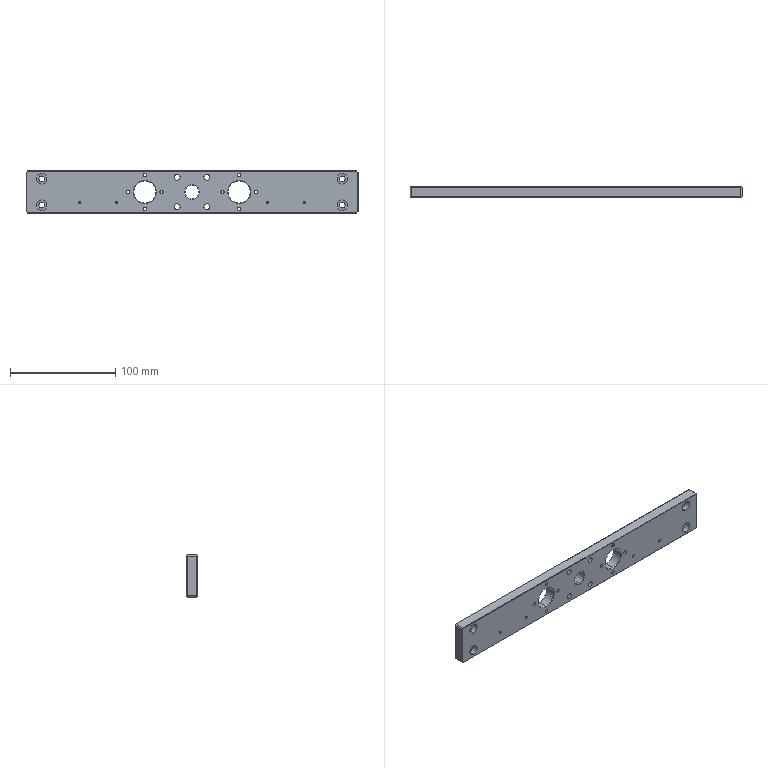Part | STEP file | PN_0022 stopper air cylinder fixing seat | 1 solid | 116 faces | box 316 x 10 x 40 mm | volume 112914 mm3 | cylinder 62 | plane 34 | cone 20 | commonest cylinder face diameters 3.3 x16 5.5 x16 10 x16 2.5 x8 21 x4 13 x2